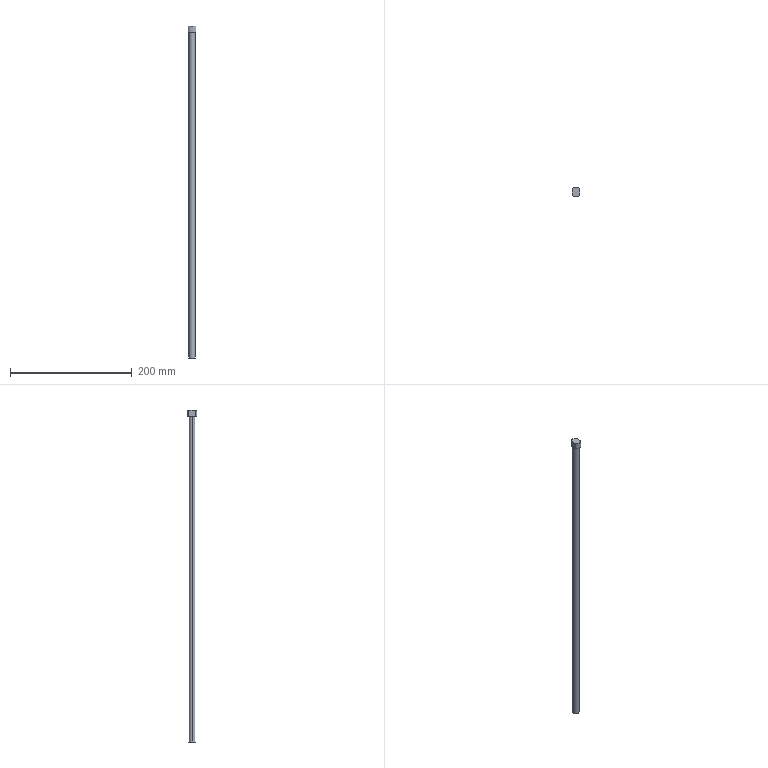Part | SolidWorks | features BaseBody 1 | 1 solid | 9 faces | box 12 x 16 x 545 mm | volume 43739 mm3 | plane 5 | cylinder 4 | commonest cylinder face diameters 10 x2 16 x2
STEP:
#1=CARTESIAN_POINT('',(-5.,0.,535.));
#2=VERTEX_POINT('',#1);
#3=CARTESIAN_POINT('',(5.,0.,535.));
#4=VERTEX_POINT('',#3);
#5=CARTESIAN_POINT('',(0.,0.,535.));
#6=DIRECTION('',(0.,0.,-1.));
#7=DIRECTION('',(-1.,0.,0.));
#8=AXIS2_PLACEMENT_3D('',#5,#6,#7);
#9=CIRCLE('',#8,5.);
#10=EDGE_CURVE('',#2,#4,#9,.T.);
#11=ORIENTED_EDGE('',*,*,#10,.T.);
#12=CARTESIAN_POINT('',(5.,0.,0.));
#13=VERTEX_POINT('',#12);
#14=CARTESIAN_POINT('',(5.,0.,535.));
#15=DIRECTION('',(0.,0.,-1.));
#16=VECTOR('',#15,1000.);
#17=LINE('',#14,#16);
#18=EDGE_CURVE('',#4,#13,#17,.T.);
#19=ORIENTED_EDGE('',*,*,#18,.T.);
#20=CARTESIAN_POINT('',(-5.,0.,0.));
#21=VERTEX_POINT('',#20);
#22=CARTESIAN_POINT('',(0.,0.,0.));
#23=DIRECTION('',(0.,0.,1.));
#24=DIRECTION('',(-1.,0.,0.));
#25=AXIS2_PLACEMENT_3D('',#22,#23,#24);
#26=CIRCLE('',#25,5.);
#27=EDGE_CURVE('',#13,#21,#26,.T.);
#28=ORIENTED_EDGE('',*,*,#27,.T.);
#29=CARTESIAN_POINT('',(-5.,0.,535.));
#30=DIRECTION('',(0.,0.,-1.));
#31=VECTOR('',#30,1000.);
#32=LINE('',#29,#31);
#33=EDGE_CURVE('',#2,#21,#32,.T.);
#34=ORIENTED_EDGE('',*,*,#33,.F.);
#35=EDGE_LOOP('',(#11,#19,#28,#34));
#36=FACE_OUTER_BOUND('',#35,.T.);
#37=CARTESIAN_POINT('',(0.,0.,535.));
#38=DIRECTION('',(0.,0.,-1.));
#39=DIRECTION('',(-1.,0.,0.));
#40=AXIS2_PLACEMENT_3D('',#37,#38,#39);
#41=CYLINDRICAL_SURFACE('',#40,5.);
#42=ADVANCED_FACE('',(#36),#41,.T.);
#43=ORIENTED_EDGE('',*,*,#18,.F.);
#44=CARTESIAN_POINT('',(0.,0.,535.));
#45=DIRECTION('',(0.,0.,-1.));
#46=DIRECTION('',(-1.,0.,0.));
#47=AXIS2_PLACEMENT_3D('',#44,#45,#46);
#48=CIRCLE('',#47,5.);
#49=EDGE_CURVE('',#4,#2,#48,.T.);
#50=ORIENTED_EDGE('',*,*,#49,.T.);
#51=ORIENTED_EDGE('',*,*,#33,.T.);
#52=CARTESIAN_POINT('',(0.,0.,0.));
#53=DIRECTION('',(0.,0.,1.));
#54=DIRECTION('',(-1.,0.,0.));
#55=AXIS2_PLACEMENT_3D('',#52,#53,#54);
#56=CIRCLE('',#55,5.);
#57=EDGE_CURVE('',#21,#13,#56,.T.);
#58=ORIENTED_EDGE('',*,*,#57,.T.);
#59=EDGE_LOOP('',(#43,#50,#51,#58));
#60=FACE_OUTER_BOUND('',#59,.T.);
#61=CARTESIAN_POINT('',(0.,0.,535.));
#62=DIRECTION('',(0.,0.,-1.));
#63=DIRECTION('',(-1.,0.,0.));
#64=AXIS2_PLACEMENT_3D('',#61,#62,#63);
#65=CYLINDRICAL_SURFACE('',#64,5.);
#66=ADVANCED_FACE('',(#60),#65,.T.);
#67=ORIENTED_EDGE('',*,*,#57,.F.);
#68=ORIENTED_EDGE('',*,*,#27,.F.);
#69=EDGE_LOOP('',(#67,#68));
#70=FACE_OUTER_BOUND('',#69,.T.);
#71=CARTESIAN_POINT('',(0.,0.,0.));
#72=DIRECTION('',(0.,0.,1.));
#73=DIRECTION('',(1.,0.,0.));
#74=AXIS2_PLACEMENT_3D('',#71,#72,#73);
#75=PLANE('',#74);
#76=ADVANCED_FACE('',(#70),#75,.F.);
#77=CARTESIAN_POINT('',(-6.,-5.292,535.));
#78=VERTEX_POINT('',#77);
#79=CARTESIAN_POINT('',(6.,-5.292,535.));
#80=VERTEX_POINT('',#79);
#81=CARTESIAN_POINT('',(0.,0.,535.));
#82=DIRECTION('',(0.,0.,1.));
#83=DIRECTION('',(-1.,0.,0.));
#84=AXIS2_PLACEMENT_3D('',#81,#82,#83);
#85=CIRCLE('',#84,8.);
#86=EDGE_CURVE('',#78,#80,#85,.T.);
#87=ORIENTED_EDGE('',*,*,#86,.F.);
#88=CARTESIAN_POINT('',(-6.,5.292,535.));
#89=VERTEX_POINT('',#88);
#90=CARTESIAN_POINT('',(-6.,0.,535.));
#91=DIRECTION('',(0.,-1.,0.));
#92=VECTOR('',#91,1000.);
#93=LINE('',#90,#92);
#94=EDGE_CURVE('',#89,#78,#93,.T.);
#95=ORIENTED_EDGE('',*,*,#94,.F.);
#96=CARTESIAN_POINT('',(6.,5.292,535.));
#97=VERTEX_POINT('',#96);
#98=CARTESIAN_POINT('',(0.,0.,535.));
#99=DIRECTION('',(0.,0.,1.));
#100=DIRECTION('',(-1.,0.,0.));
#101=AXIS2_PLACEMENT_3D('',#98,#99,#100);
#102=CIRCLE('',#101,8.);
#103=EDGE_CURVE('',#97,#89,#102,.T.);
#104=ORIENTED_EDGE('',*,*,#103,.F.);
#105=CARTESIAN_POINT('',(6.,0.,535.));
#106=DIRECTION('',(0.,1.,0.));
#107=VECTOR('',#106,1000.);
#108=LINE('',#105,#107);
#109=EDGE_CURVE('',#80,#97,#108,.T.);
#110=ORIENTED_EDGE('',*,*,#109,.F.);
#111=EDGE_LOOP('',(#87,#95,#104,#110));
#112=FACE_OUTER_BOUND('',#111,.T.);
#113=ORIENTED_EDGE('',*,*,#10,.F.);
#114=ORIENTED_EDGE('',*,*,#49,.F.);
#115=EDGE_LOOP('',(#113,#114));
#116=FACE_BOUND('',#115,.T.);
#117=CARTESIAN_POINT('',(0.,0.,535.));
#118=DIRECTION('',(0.,0.,1.));
#119=DIRECTION('',(1.,0.,0.));
#120=AXIS2_PLACEMENT_3D('',#117,#118,#119);
#121=PLANE('',#120);
#122=ADVANCED_FACE('',(#112,#116),#121,.F.);
#123=CARTESIAN_POINT('',(6.,5.292,545.));
#124=VERTEX_POINT('',#123);
#125=CARTESIAN_POINT('',(6.,5.292,535.));
#126=DIRECTION('',(0.,0.,1.));
#127=VECTOR('',#126,1000.);
#128=LINE('',#125,#127);
#129=EDGE_CURVE('',#97,#124,#128,.T.);
#130=ORIENTED_EDGE('',*,*,#129,.T.);
#131=CARTESIAN_POINT('',(6.,-5.292,545.));
#132=VERTEX_POINT('',#131);
#133=CARTESIAN_POINT('',(6.,-12.632,545.));
#134=DIRECTION('',(0.,-1.,0.));
#135=VECTOR('',#134,1000.);
#136=LINE('',#133,#135);
#137=EDGE_CURVE('',#124,#132,#136,.T.);
#138=ORIENTED_EDGE('',*,*,#137,.T.);
#139=CARTESIAN_POINT('',(6.,-5.292,535.));
#140=DIRECTION('',(0.,0.,-1.));
#141=VECTOR('',#140,1000.);
#142=LINE('',#139,#141);
#143=EDGE_CURVE('',#132,#80,#142,.T.);
#144=ORIENTED_EDGE('',*,*,#143,.T.);
#145=ORIENTED_EDGE('',*,*,#109,.T.);
#146=EDGE_LOOP('',(#130,#138,#144,#145));
#147=FACE_OUTER_BOUND('',#146,.T.);
#148=CARTESIAN_POINT('',(6.,-12.632,535.));
#149=DIRECTION('',(1.,0.,0.));
#150=DIRECTION('',(0.,0.,-1.));
#151=AXIS2_PLACEMENT_3D('',#148,#149,#150);
#152=PLANE('',#151);
#153=ADVANCED_FACE('',(#147),#152,.T.);
#154=CARTESIAN_POINT('',(-6.,-5.292,545.));
#155=VERTEX_POINT('',#154);
#156=CARTESIAN_POINT('',(-6.,-5.292,545.));
#157=DIRECTION('',(0.,0.,-1.));
#158=VECTOR('',#157,1000.);
#159=LINE('',#156,#158);
#160=EDGE_CURVE('',#155,#78,#159,.T.);
#161=ORIENTED_EDGE('',*,*,#160,.T.);
#162=ORIENTED_EDGE('',*,*,#86,.T.);
#163=ORIENTED_EDGE('',*,*,#143,.F.);
#164=CARTESIAN_POINT('',(0.,0.,545.));
#165=DIRECTION('',(0.,0.,-1.));
#166=DIRECTION('',(-1.,0.,0.));
#167=AXIS2_PLACEMENT_3D('',#164,#165,#166);
#168=CIRCLE('',#167,8.);
#169=EDGE_CURVE('',#132,#155,#168,.T.);
#170=ORIENTED_EDGE('',*,*,#169,.T.);
#171=EDGE_LOOP('',(#161,#162,#163,#170));
#172=FACE_OUTER_BOUND('',#171,.T.);
#173=CARTESIAN_POINT('',(0.,0.,545.));
#174=DIRECTION('',(0.,0.,-1.));
#175=DIRECTION('',(-1.,0.,0.));
#176=AXIS2_PLACEMENT_3D('',#173,#174,#175);
#177=CYLINDRICAL_SURFACE('',#176,8.);
#178=ADVANCED_FACE('',(#172),#177,.T.);
#179=ORIENTED_EDGE('',*,*,#160,.F.);
#180=CARTESIAN_POINT('',(-6.,5.292,545.));
#181=VERTEX_POINT('',#180);
#182=CARTESIAN_POINT('',(-6.,-12.632,545.));
#183=DIRECTION('',(0.,1.,0.));
#184=VECTOR('',#183,1000.);
#185=LINE('',#182,#184);
#186=EDGE_CURVE('',#155,#181,#185,.T.);
#187=ORIENTED_EDGE('',*,*,#186,.T.);
#188=CARTESIAN_POINT('',(-6.,5.292,535.));
#189=DIRECTION('',(0.,0.,-1.));
#190=VECTOR('',#189,1000.);
#191=LINE('',#188,#190);
#192=EDGE_CURVE('',#181,#89,#191,.T.);
#193=ORIENTED_EDGE('',*,*,#192,.T.);
#194=ORIENTED_EDGE('',*,*,#94,.T.);
#195=EDGE_LOOP('',(#179,#187,#193,#194));
#196=FACE_OUTER_BOUND('',#195,.T.);
#197=CARTESIAN_POINT('',(-6.,-12.632,535.));
#198=DIRECTION('',(-1.,0.,0.));
#199=DIRECTION('',(0.,0.,1.));
#200=AXIS2_PLACEMENT_3D('',#197,#198,#199);
#201=PLANE('',#200);
#202=ADVANCED_FACE('',(#196),#201,.T.);
#203=ORIENTED_EDGE('',*,*,#192,.F.);
#204=CARTESIAN_POINT('',(0.,0.,545.));
#205=DIRECTION('',(0.,0.,-1.));
#206=DIRECTION('',(-1.,0.,0.));
#207=AXIS2_PLACEMENT_3D('',#204,#205,#206);
#208=CIRCLE('',#207,8.);
#209=EDGE_CURVE('',#181,#124,#208,.T.);
#210=ORIENTED_EDGE('',*,*,#209,.T.);
#211=ORIENTED_EDGE('',*,*,#129,.F.);
#212=ORIENTED_EDGE('',*,*,#103,.T.);
#213=EDGE_LOOP('',(#203,#210,#211,#212));
#214=FACE_OUTER_BOUND('',#213,.T.);
#215=CARTESIAN_POINT('',(0.,0.,545.));
#216=DIRECTION('',(0.,0.,-1.));
#217=DIRECTION('',(-1.,0.,0.));
#218=AXIS2_PLACEMENT_3D('',#215,#216,#217);
#219=CYLINDRICAL_SURFACE('',#218,8.);
#220=ADVANCED_FACE('',(#214),#219,.T.);
#221=ORIENTED_EDGE('',*,*,#209,.F.);
#222=ORIENTED_EDGE('',*,*,#186,.F.);
#223=ORIENTED_EDGE('',*,*,#169,.F.);
#224=ORIENTED_EDGE('',*,*,#137,.F.);
#225=EDGE_LOOP('',(#221,#222,#223,#224));
#226=FACE_OUTER_BOUND('',#225,.T.);
#227=CARTESIAN_POINT('',(0.,0.,545.));
#228=DIRECTION('',(0.,0.,1.));
#229=DIRECTION('',(1.,0.,0.));
#230=AXIS2_PLACEMENT_3D('',#227,#228,#229);
#231=PLANE('',#230);
#232=ADVANCED_FACE('',(#226),#231,.T.);
#233=CLOSED_SHELL('',(#42,#66,#76,#122,#153,#178,#202,#220,#232));
#234=MANIFOLD_SOLID_BREP('',#233);
#235=CARTESIAN_POINT('',(0.,0.,0.));
#236=DIRECTION('',(0.,0.,1.));
#237=DIRECTION('',(1.,0.,0.));
#238=AXIS2_PLACEMENT_3D('',#235,#236,#237);
#239=(LENGTH_UNIT()NAMED_UNIT(*)SI_UNIT(.MILLI.,.METRE.));
#240=UNCERTAINTY_MEASURE_WITH_UNIT(LENGTH_MEASURE(0.00001),#239,'','');
#241=(NAMED_UNIT(*)PLANE_ANGLE_UNIT()SI_UNIT($,.RADIAN.));
#242=(NAMED_UNIT(*)SI_UNIT($,.STERADIAN.)SOLID_ANGLE_UNIT());
#243=(GEOMETRIC_REPRESENTATION_CONTEXT(3)GLOBAL_UNCERTAINTY_ASSIGNED_CONTEXT((#240))GLOBAL_UNIT_ASSIGNED_CONTEXT((#239,#241,#242))REPRESENTATION_CONTEXT('',''));
#244=ADVANCED_BREP_SHAPE_REPRESENTATION('',(#234,#238),#243);